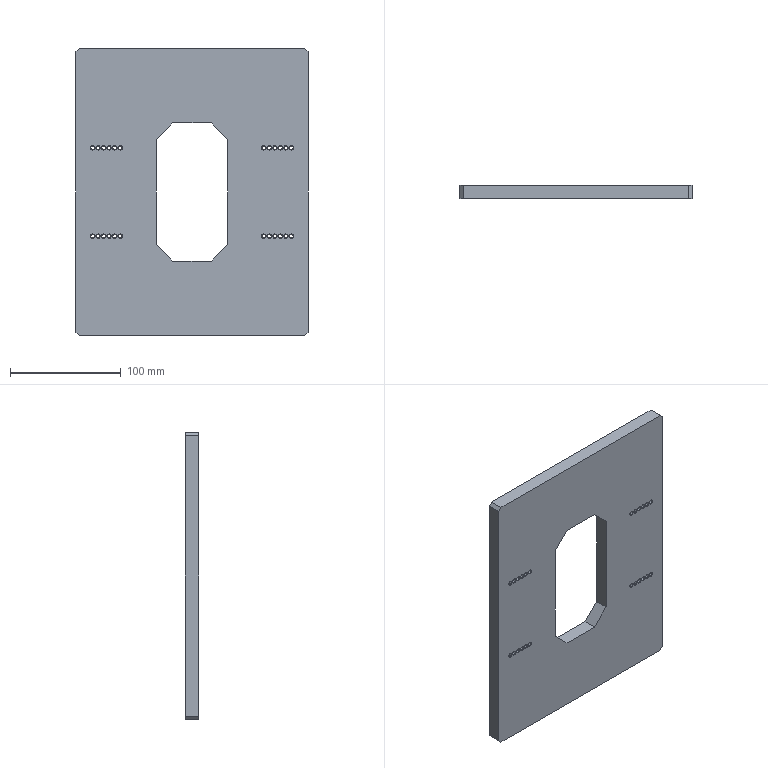Part | SolidWorks | features Chamfer 2, MirrorPattern 2, 3DProfileFeature 1, Extrusion 1, HoleWzd 1, ICE 1, LPattern 1 | 1 solid | 114 faces | box 210 x 12 x 260 mm | volume 560402 mm3 | cone 48 | cylinder 48 | plane 18 | commonest cylinder face diameters 3.3 x48